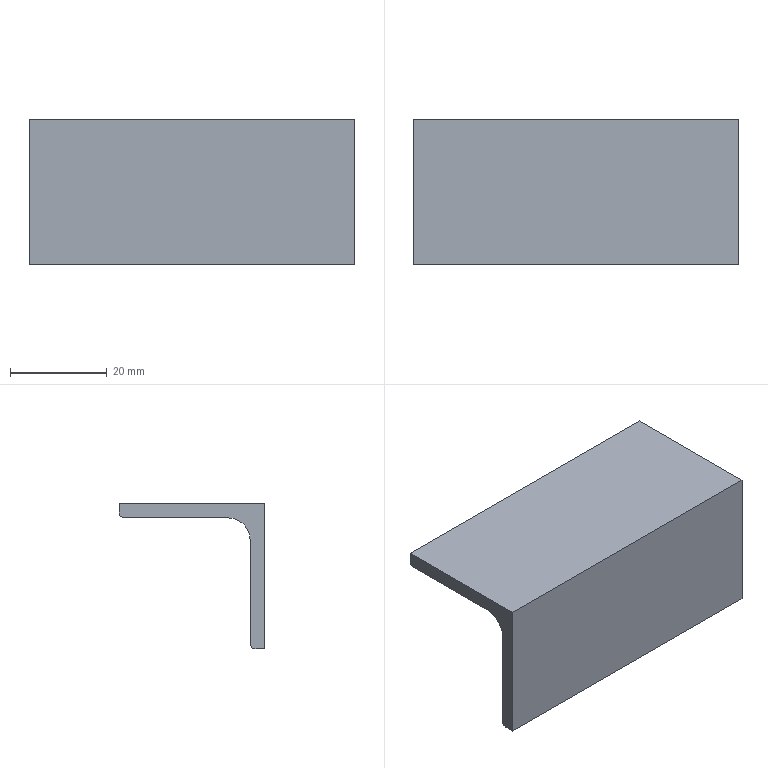Part | STEP file | 02-Angle steel 30x30x3_default<machining> | 1 solid | 11 faces | box 67 x 30 x 30 mm | volume 11719 mm3 | plane 8 | cylinder 3 | commonest cylinder face diameters 2 x2 9 x1
STEP:
#1=CARTESIAN_POINT('',(0.,0.,0.));
#2=DIRECTION('',(0.,0.,1.));
#3=DIRECTION('',(1.,0.,0.));
#4=AXIS2_PLACEMENT_3D('',#1,#2,#3);
#5=CARTESIAN_POINT('',(0.,30.,-2.));
#6=VERTEX_POINT('',#5);
#7=CARTESIAN_POINT('',(0.,30.,0.));
#8=VERTEX_POINT('',#7);
#9=CARTESIAN_POINT('',(0.,30.,0.));
#10=DIRECTION('',(0.,0.,1.));
#11=VECTOR('',#10,1.);
#12=LINE('',#9,#11);
#13=CARTESIAN_POINT('',(67.,30.,0.));
#14=DIRECTION('',(0.,-1.,0.));
#15=DIRECTION('',(0.,0.,-1.));
#16=AXIS2_PLACEMENT_3D('',#13,#14,#15);
#17=PLANE('',#16);
#18=CARTESIAN_POINT('',(0.,-67.));
#19=DIRECTION('',(-1.,0.));
#20=VECTOR('',#19,1.);
#21=LINE('',#18,#20);
#22=(GEOMETRIC_REPRESENTATION_CONTEXT(2)PARAMETRIC_REPRESENTATION_CONTEXT()REPRESENTATION_CONTEXT('',''));
#23=DEFINITIONAL_REPRESENTATION('',(#21),#22);
#24=PCURVE('',#17,#23);
#25=CARTESIAN_POINT('',(0.,29.,-2.));
#26=DIRECTION('',(-1.,0.,0.));
#27=DIRECTION('',(0.,0.,1.));
#28=AXIS2_PLACEMENT_3D('',#25,#26,#27);
#29=PLANE('',#28);
#30=CARTESIAN_POINT('',(2.,1.));
#31=DIRECTION('',(1.,0.));
#32=VECTOR('',#31,1.);
#33=LINE('',#30,#32);
#34=(GEOMETRIC_REPRESENTATION_CONTEXT(2)PARAMETRIC_REPRESENTATION_CONTEXT()REPRESENTATION_CONTEXT('',''));
#35=DEFINITIONAL_REPRESENTATION('',(#33),#34);
#36=PCURVE('',#29,#35);
#37=SURFACE_CURVE('',#12,(#24,#36),.PCURVE_S1.);
#38=EDGE_CURVE('',#6,#8,#37,.T.);
#39=ORIENTED_EDGE('',*,*,#38,.T.);
#40=CARTESIAN_POINT('',(67.,30.,0.));
#41=VERTEX_POINT('',#40);
#42=CARTESIAN_POINT('',(67.,30.,0.));
#43=DIRECTION('',(-1.,0.,0.));
#44=VECTOR('',#43,1.);
#45=LINE('',#42,#44);
#46=CARTESIAN_POINT('',(0.,0.));
#47=DIRECTION('',(0.,-1.));
#48=VECTOR('',#47,1.);
#49=LINE('',#46,#48);
#50=(GEOMETRIC_REPRESENTATION_CONTEXT(2)PARAMETRIC_REPRESENTATION_CONTEXT()REPRESENTATION_CONTEXT('',''));
#51=DEFINITIONAL_REPRESENTATION('',(#49),#50);
#52=PCURVE('',#17,#51);
#53=CARTESIAN_POINT('',(67.,30.,0.));
#54=DIRECTION('',(0.,0.,-1.));
#55=DIRECTION('',(0.,1.,0.));
#56=AXIS2_PLACEMENT_3D('',#53,#54,#55);
#57=PLANE('',#56);
#58=CARTESIAN_POINT('',(0.,0.));
#59=DIRECTION('',(0.,-1.));
#60=VECTOR('',#59,1.);
#61=LINE('',#58,#60);
#62=(GEOMETRIC_REPRESENTATION_CONTEXT(2)PARAMETRIC_REPRESENTATION_CONTEXT()REPRESENTATION_CONTEXT('',''));
#63=DEFINITIONAL_REPRESENTATION('',(#61),#62);
#64=PCURVE('',#57,#63);
#65=SURFACE_CURVE('',#45,(#52,#64),.PCURVE_S1.);
#66=EDGE_CURVE('',#41,#8,#65,.T.);
#67=ORIENTED_EDGE('',*,*,#66,.F.);
#68=CARTESIAN_POINT('',(67.,30.,-2.));
#69=VERTEX_POINT('',#68);
#70=CARTESIAN_POINT('',(67.,30.,0.));
#71=DIRECTION('',(0.,0.,1.));
#72=VECTOR('',#71,1.);
#73=LINE('',#70,#72);
#74=CARTESIAN_POINT('',(0.,0.));
#75=DIRECTION('',(-1.,0.));
#76=VECTOR('',#75,1.);
#77=LINE('',#74,#76);
#78=(GEOMETRIC_REPRESENTATION_CONTEXT(2)PARAMETRIC_REPRESENTATION_CONTEXT()REPRESENTATION_CONTEXT('',''));
#79=DEFINITIONAL_REPRESENTATION('',(#77),#78);
#80=PCURVE('',#17,#79);
#81=CARTESIAN_POINT('',(67.,29.,-2.));
#82=DIRECTION('',(-1.,0.,0.));
#83=DIRECTION('',(0.,0.,1.));
#84=AXIS2_PLACEMENT_3D('',#81,#82,#83);
#85=PLANE('',#84);
#86=CARTESIAN_POINT('',(2.,1.));
#87=DIRECTION('',(1.,0.));
#88=VECTOR('',#87,1.);
#89=LINE('',#86,#88);
#90=(GEOMETRIC_REPRESENTATION_CONTEXT(2)PARAMETRIC_REPRESENTATION_CONTEXT()REPRESENTATION_CONTEXT('',''));
#91=DEFINITIONAL_REPRESENTATION('',(#89),#90);
#92=PCURVE('',#85,#91);
#93=SURFACE_CURVE('',#73,(#80,#92),.PCURVE_S1.);
#94=EDGE_CURVE('',#69,#41,#93,.T.);
#95=ORIENTED_EDGE('',*,*,#94,.F.);
#96=CARTESIAN_POINT('',(67.,30.,-2.));
#97=DIRECTION('',(-1.,0.,0.));
#98=VECTOR('',#97,1.);
#99=LINE('',#96,#98);
#100=CARTESIAN_POINT('',(2.,0.));
#101=DIRECTION('',(0.,-1.));
#102=VECTOR('',#101,1.);
#103=LINE('',#100,#102);
#104=(GEOMETRIC_REPRESENTATION_CONTEXT(2)PARAMETRIC_REPRESENTATION_CONTEXT()REPRESENTATION_CONTEXT('',''));
#105=DEFINITIONAL_REPRESENTATION('',(#103),#104);
#106=PCURVE('',#17,#105);
#107=CARTESIAN_POINT('',(67.,29.,-2.));
#108=DIRECTION('',(-1.,0.,0.));
#109=DIRECTION('',(0.,0.,1.));
#110=AXIS2_PLACEMENT_3D('',#107,#108,#109);
#111=CYLINDRICAL_SURFACE('',#110,1.);
#112=CARTESIAN_POINT('',(1.571,0.));
#113=DIRECTION('',(0.,1.));
#114=VECTOR('',#113,1.);
#115=LINE('',#112,#114);
#116=(GEOMETRIC_REPRESENTATION_CONTEXT(2)PARAMETRIC_REPRESENTATION_CONTEXT()REPRESENTATION_CONTEXT('',''));
#117=DEFINITIONAL_REPRESENTATION('',(#115),#116);
#118=PCURVE('',#111,#117);
#119=SURFACE_CURVE('',#99,(#106,#118),.PCURVE_S1.);
#120=EDGE_CURVE('',#69,#6,#119,.T.);
#121=ORIENTED_EDGE('',*,*,#120,.T.);
#122=EDGE_LOOP('',(#39,#67,#95,#121));
#123=FACE_BOUND('',#122,.T.);
#124=ADVANCED_FACE('',(#123),#17,.F.);
#125=CARTESIAN_POINT('',(0.,0.,0.));
#126=VERTEX_POINT('',#125);
#127=CARTESIAN_POINT('',(0.,30.,0.));
#128=DIRECTION('',(0.,-1.,0.));
#129=VECTOR('',#128,1.);
#130=LINE('',#127,#129);
#131=CARTESIAN_POINT('',(0.,-67.));
#132=DIRECTION('',(-1.,0.));
#133=VECTOR('',#132,1.);
#134=LINE('',#131,#133);
#135=(GEOMETRIC_REPRESENTATION_CONTEXT(2)PARAMETRIC_REPRESENTATION_CONTEXT()REPRESENTATION_CONTEXT('',''));
#136=DEFINITIONAL_REPRESENTATION('',(#134),#135);
#137=PCURVE('',#57,#136);
#138=CARTESIAN_POINT('',(2.,1.));
#139=DIRECTION('',(0.,-1.));
#140=VECTOR('',#139,1.);
#141=LINE('',#138,#140);
#142=(GEOMETRIC_REPRESENTATION_CONTEXT(2)PARAMETRIC_REPRESENTATION_CONTEXT()REPRESENTATION_CONTEXT('',''));
#143=DEFINITIONAL_REPRESENTATION('',(#141),#142);
#144=PCURVE('',#29,#143);
#145=SURFACE_CURVE('',#130,(#137,#144),.PCURVE_S1.);
#146=EDGE_CURVE('',#8,#126,#145,.T.);
#147=ORIENTED_EDGE('',*,*,#146,.T.);
#148=CARTESIAN_POINT('',(67.,0.,0.));
#149=VERTEX_POINT('',#148);
#150=CARTESIAN_POINT('',(67.,0.,0.));
#151=DIRECTION('',(-1.,0.,0.));
#152=VECTOR('',#151,1.);
#153=LINE('',#150,#152);
#154=CARTESIAN_POINT('',(-30.,0.));
#155=DIRECTION('',(0.,-1.));
#156=VECTOR('',#155,1.);
#157=LINE('',#154,#156);
#158=(GEOMETRIC_REPRESENTATION_CONTEXT(2)PARAMETRIC_REPRESENTATION_CONTEXT()REPRESENTATION_CONTEXT('',''));
#159=DEFINITIONAL_REPRESENTATION('',(#157),#158);
#160=PCURVE('',#57,#159);
#161=CARTESIAN_POINT('',(67.,0.,0.));
#162=DIRECTION('',(0.,1.,0.));
#163=DIRECTION('',(0.,0.,1.));
#164=AXIS2_PLACEMENT_3D('',#161,#162,#163);
#165=PLANE('',#164);
#166=CARTESIAN_POINT('',(0.,0.));
#167=DIRECTION('',(0.,-1.));
#168=VECTOR('',#167,1.);
#169=LINE('',#166,#168);
#170=(GEOMETRIC_REPRESENTATION_CONTEXT(2)PARAMETRIC_REPRESENTATION_CONTEXT()REPRESENTATION_CONTEXT('',''));
#171=DEFINITIONAL_REPRESENTATION('',(#169),#170);
#172=PCURVE('',#165,#171);
#173=SURFACE_CURVE('',#153,(#160,#172),.PCURVE_S1.);
#174=EDGE_CURVE('',#149,#126,#173,.T.);
#175=ORIENTED_EDGE('',*,*,#174,.F.);
#176=CARTESIAN_POINT('',(67.,30.,0.));
#177=DIRECTION('',(0.,-1.,0.));
#178=VECTOR('',#177,1.);
#179=LINE('',#176,#178);
#180=CARTESIAN_POINT('',(0.,0.));
#181=DIRECTION('',(-1.,0.));
#182=VECTOR('',#181,1.);
#183=LINE('',#180,#182);
#184=(GEOMETRIC_REPRESENTATION_CONTEXT(2)PARAMETRIC_REPRESENTATION_CONTEXT()REPRESENTATION_CONTEXT('',''));
#185=DEFINITIONAL_REPRESENTATION('',(#183),#184);
#186=PCURVE('',#57,#185);
#187=CARTESIAN_POINT('',(2.,1.));
#188=DIRECTION('',(0.,-1.));
#189=VECTOR('',#188,1.);
#190=LINE('',#187,#189);
#191=(GEOMETRIC_REPRESENTATION_CONTEXT(2)PARAMETRIC_REPRESENTATION_CONTEXT()REPRESENTATION_CONTEXT('',''));
#192=DEFINITIONAL_REPRESENTATION('',(#190),#191);
#193=PCURVE('',#85,#192);
#194=SURFACE_CURVE('',#179,(#186,#193),.PCURVE_S1.);
#195=EDGE_CURVE('',#41,#149,#194,.T.);
#196=ORIENTED_EDGE('',*,*,#195,.F.);
#197=ORIENTED_EDGE('',*,*,#66,.T.);
#198=EDGE_LOOP('',(#147,#175,#196,#197));
#199=FACE_BOUND('',#198,.T.);
#200=ADVANCED_FACE('',(#199),#57,.F.);
#201=CARTESIAN_POINT('',(0.,0.,-30.));
#202=VERTEX_POINT('',#201);
#203=CARTESIAN_POINT('',(0.,0.,0.));
#204=DIRECTION('',(0.,0.,-1.));
#205=VECTOR('',#204,1.);
#206=LINE('',#203,#205);
#207=CARTESIAN_POINT('',(0.,-67.));
#208=DIRECTION('',(-1.,0.));
#209=VECTOR('',#208,1.);
#210=LINE('',#207,#209);
#211=(GEOMETRIC_REPRESENTATION_CONTEXT(2)PARAMETRIC_REPRESENTATION_CONTEXT()REPRESENTATION_CONTEXT('',''));
#212=DEFINITIONAL_REPRESENTATION('',(#210),#211);
#213=PCURVE('',#165,#212);
#214=CARTESIAN_POINT('',(2.,-29.));
#215=DIRECTION('',(-1.,0.));
#216=VECTOR('',#215,1.);
#217=LINE('',#214,#216);
#218=(GEOMETRIC_REPRESENTATION_CONTEXT(2)PARAMETRIC_REPRESENTATION_CONTEXT()REPRESENTATION_CONTEXT('',''));
#219=DEFINITIONAL_REPRESENTATION('',(#217),#218);
#220=PCURVE('',#29,#219);
#221=SURFACE_CURVE('',#206,(#213,#220),.PCURVE_S1.);
#222=EDGE_CURVE('',#126,#202,#221,.T.);
#223=ORIENTED_EDGE('',*,*,#222,.T.);
#224=CARTESIAN_POINT('',(67.,0.,-30.));
#225=VERTEX_POINT('',#224);
#226=CARTESIAN_POINT('',(67.,0.,-30.));
#227=DIRECTION('',(-1.,0.,0.));
#228=VECTOR('',#227,1.);
#229=LINE('',#226,#228);
#230=CARTESIAN_POINT('',(-30.,0.));
#231=DIRECTION('',(0.,-1.));
#232=VECTOR('',#231,1.);
#233=LINE('',#230,#232);
#234=(GEOMETRIC_REPRESENTATION_CONTEXT(2)PARAMETRIC_REPRESENTATION_CONTEXT()REPRESENTATION_CONTEXT('',''));
#235=DEFINITIONAL_REPRESENTATION('',(#233),#234);
#236=PCURVE('',#165,#235);
#237=CARTESIAN_POINT('',(67.,0.,-30.));
#238=DIRECTION('',(0.,0.,1.));
#239=DIRECTION('',(0.,-1.,0.));
#240=AXIS2_PLACEMENT_3D('',#237,#238,#239);
#241=PLANE('',#240);
#242=CARTESIAN_POINT('',(0.,0.));
#243=DIRECTION('',(0.,-1.));
#244=VECTOR('',#243,1.);
#245=LINE('',#242,#244);
#246=(GEOMETRIC_REPRESENTATION_CONTEXT(2)PARAMETRIC_REPRESENTATION_CONTEXT()REPRESENTATION_CONTEXT('',''));
#247=DEFINITIONAL_REPRESENTATION('',(#245),#246);
#248=PCURVE('',#241,#247);
#249=SURFACE_CURVE('',#229,(#236,#248),.PCURVE_S1.);
#250=EDGE_CURVE('',#225,#202,#249,.T.);
#251=ORIENTED_EDGE('',*,*,#250,.F.);
#252=CARTESIAN_POINT('',(67.,0.,0.));
#253=DIRECTION('',(0.,0.,-1.));
#254=VECTOR('',#253,1.);
#255=LINE('',#252,#254);
#256=CARTESIAN_POINT('',(0.,0.));
#257=DIRECTION('',(-1.,0.));
#258=VECTOR('',#257,1.);
#259=LINE('',#256,#258);
#260=(GEOMETRIC_REPRESENTATION_CONTEXT(2)PARAMETRIC_REPRESENTATION_CONTEXT()REPRESENTATION_CONTEXT('',''));
#261=DEFINITIONAL_REPRESENTATION('',(#259),#260);
#262=PCURVE('',#165,#261);
#263=CARTESIAN_POINT('',(2.,-29.));
#264=DIRECTION('',(-1.,0.));
#265=VECTOR('',#264,1.);
#266=LINE('',#263,#265);
#267=(GEOMETRIC_REPRESENTATION_CONTEXT(2)PARAMETRIC_REPRESENTATION_CONTEXT()REPRESENTATION_CONTEXT('',''));
#268=DEFINITIONAL_REPRESENTATION('',(#266),#267);
#269=PCURVE('',#85,#268);
#270=SURFACE_CURVE('',#255,(#262,#269),.PCURVE_S1.);
#271=EDGE_CURVE('',#149,#225,#270,.T.);
#272=ORIENTED_EDGE('',*,*,#271,.F.);
#273=ORIENTED_EDGE('',*,*,#174,.T.);
#274=EDGE_LOOP('',(#223,#251,#272,#273));
#275=FACE_BOUND('',#274,.T.);
#276=ADVANCED_FACE('',(#275),#165,.F.);
#277=CARTESIAN_POINT('',(0.,2.,-30.));
#278=VERTEX_POINT('',#277);
#279=CARTESIAN_POINT('',(0.,0.,-30.));
#280=DIRECTION('',(0.,1.,0.));
#281=VECTOR('',#280,1.);
#282=LINE('',#279,#281);
#283=CARTESIAN_POINT('',(0.,-67.));
#284=DIRECTION('',(-1.,0.));
#285=VECTOR('',#284,1.);
#286=LINE('',#283,#285);
#287=(GEOMETRIC_REPRESENTATION_CONTEXT(2)PARAMETRIC_REPRESENTATION_CONTEXT()REPRESENTATION_CONTEXT('',''));
#288=DEFINITIONAL_REPRESENTATION('',(#286),#287);
#289=PCURVE('',#241,#288);
#290=CARTESIAN_POINT('',(-28.,-29.));
#291=DIRECTION('',(0.,1.));
#292=VECTOR('',#291,1.);
#293=LINE('',#290,#292);
#294=(GEOMETRIC_REPRESENTATION_CONTEXT(2)PARAMETRIC_REPRESENTATION_CONTEXT()REPRESENTATION_CONTEXT('',''));
#295=DEFINITIONAL_REPRESENTATION('',(#293),#294);
#296=PCURVE('',#29,#295);
#297=SURFACE_CURVE('',#282,(#289,#296),.PCURVE_S1.);
#298=EDGE_CURVE('',#202,#278,#297,.T.);
#299=ORIENTED_EDGE('',*,*,#298,.T.);
#300=CARTESIAN_POINT('',(67.,2.,-30.));
#301=VERTEX_POINT('',#300);
#302=CARTESIAN_POINT('',(67.,2.,-30.));
#303=DIRECTION('',(-1.,0.,0.));
#304=VECTOR('',#303,1.);
#305=LINE('',#302,#304);
#306=CARTESIAN_POINT('',(-2.,0.));
#307=DIRECTION('',(0.,-1.));
#308=VECTOR('',#307,1.);
#309=LINE('',#306,#308);
#310=(GEOMETRIC_REPRESENTATION_CONTEXT(2)PARAMETRIC_REPRESENTATION_CONTEXT()REPRESENTATION_CONTEXT('',''));
#311=DEFINITIONAL_REPRESENTATION('',(#309),#310);
#312=PCURVE('',#241,#311);
#313=CARTESIAN_POINT('',(67.,2.,-29.));
#314=DIRECTION('',(-1.,0.,0.));
#315=DIRECTION('',(0.,0.,1.));
#316=AXIS2_PLACEMENT_3D('',#313,#314,#315);
#317=CYLINDRICAL_SURFACE('',#316,1.);
#318=CARTESIAN_POINT('',(3.142,0.));
#319=DIRECTION('',(0.,1.));
#320=VECTOR('',#319,1.);
#321=LINE('',#318,#320);
#322=(GEOMETRIC_REPRESENTATION_CONTEXT(2)PARAMETRIC_REPRESENTATION_CONTEXT()REPRESENTATION_CONTEXT('',''));
#323=DEFINITIONAL_REPRESENTATION('',(#321),#322);
#324=PCURVE('',#317,#323);
#325=SURFACE_CURVE('',#305,(#312,#324),.PCURVE_S1.);
#326=EDGE_CURVE('',#301,#278,#325,.T.);
#327=ORIENTED_EDGE('',*,*,#326,.F.);
#328=CARTESIAN_POINT('',(67.,0.,-30.));
#329=DIRECTION('',(0.,1.,0.));
#330=VECTOR('',#329,1.);
#331=LINE('',#328,#330);
#332=CARTESIAN_POINT('',(0.,0.));
#333=DIRECTION('',(-1.,0.));
#334=VECTOR('',#333,1.);
#335=LINE('',#332,#334);
#336=(GEOMETRIC_REPRESENTATION_CONTEXT(2)PARAMETRIC_REPRESENTATION_CONTEXT()REPRESENTATION_CONTEXT('',''));
#337=DEFINITIONAL_REPRESENTATION('',(#335),#336);
#338=PCURVE('',#241,#337);
#339=CARTESIAN_POINT('',(-28.,-29.));
#340=DIRECTION('',(0.,1.));
#341=VECTOR('',#340,1.);
#342=LINE('',#339,#341);
#343=(GEOMETRIC_REPRESENTATION_CONTEXT(2)PARAMETRIC_REPRESENTATION_CONTEXT()REPRESENTATION_CONTEXT('',''));
#344=DEFINITIONAL_REPRESENTATION('',(#342),#343);
#345=PCURVE('',#85,#344);
#346=SURFACE_CURVE('',#331,(#338,#345),.PCURVE_S1.);
#347=EDGE_CURVE('',#225,#301,#346,.T.);
#348=ORIENTED_EDGE('',*,*,#347,.F.);
#349=ORIENTED_EDGE('',*,*,#250,.T.);
#350=EDGE_LOOP('',(#299,#327,#348,#349));
#351=FACE_BOUND('',#350,.T.);
#352=ADVANCED_FACE('',(#351),#241,.F.);
#353=CARTESIAN_POINT('',(0.,3.,-29.));
#354=VERTEX_POINT('',#353);
#355=CARTESIAN_POINT('',(0.,2.,-29.));
#356=DIRECTION('',(1.,0.,0.));
#357=DIRECTION('',(0.,0.,-1.));
#358=AXIS2_PLACEMENT_3D('',#355,#356,#357);
#359=CIRCLE('',#358,1.);
#360=CARTESIAN_POINT('',(3.142,67.));
#361=DIRECTION('',(-1.,0.));
#362=VECTOR('',#361,1.);
#363=LINE('',#360,#362);
#364=(GEOMETRIC_REPRESENTATION_CONTEXT(2)PARAMETRIC_REPRESENTATION_CONTEXT()REPRESENTATION_CONTEXT('',''));
#365=DEFINITIONAL_REPRESENTATION('',(#363),#364);
#366=PCURVE('',#317,#365);
#367=CARTESIAN_POINT('',(-28.,-27.));
#368=CARTESIAN_POINT('',(-28.,-25.268));
#369=CARTESIAN_POINT('',(-26.5,-26.134));
#370=CARTESIAN_POINT('',(-25.,-27.));
#371=CARTESIAN_POINT('',(-26.5,-27.866));
#372=CARTESIAN_POINT('',(-28.,-28.732));
#373=CARTESIAN_POINT('',(-28.,-27.));
#374=(BOUNDED_CURVE()B_SPLINE_CURVE(2,(#367,#368,#369,#370,#371,#372,#373),.UNSPECIFIED.,.T.,.F.)B_SPLINE_CURVE_WITH_KNOTS((1,2,2,2,2,1),(-2.094,0.,2.094,4.189,6.283,8.378),.UNSPECIFIED.)CURVE()GEOMETRIC_REPRESENTATION_ITEM()RATIONAL_B_SPLINE_CURVE((1.,0.5,1.,0.5,1.,0.5,1.))REPRESENTATION_ITEM(''));
#375=(GEOMETRIC_REPRESENTATION_CONTEXT(2)PARAMETRIC_REPRESENTATION_CONTEXT()REPRESENTATION_CONTEXT('',''));
#376=DEFINITIONAL_REPRESENTATION('',(#374),#375);
#377=PCURVE('',#29,#376);
#378=SURFACE_CURVE('',#359,(#366,#377),.PCURVE_S1.);
#379=EDGE_CURVE('',#278,#354,#378,.T.);
#380=ORIENTED_EDGE('',*,*,#379,.T.);
#381=CARTESIAN_POINT('',(67.,3.,-29.));
#382=VERTEX_POINT('',#381);
#383=CARTESIAN_POINT('',(67.,3.,-29.));
#384=DIRECTION('',(-1.,0.,0.));
#385=VECTOR('',#384,1.);
#386=LINE('',#383,#385);
#387=CARTESIAN_POINT('',(1.571,0.));
#388=DIRECTION('',(0.,1.));
#389=VECTOR('',#388,1.);
#390=LINE('',#387,#389);
#391=(GEOMETRIC_REPRESENTATION_CONTEXT(2)PARAMETRIC_REPRESENTATION_CONTEXT()REPRESENTATION_CONTEXT('',''));
#392=DEFINITIONAL_REPRESENTATION('',(#390),#391);
#393=PCURVE('',#317,#392);
#394=CARTESIAN_POINT('',(67.,3.,-7.5));
#395=DIRECTION('',(0.,-1.,0.));
#396=DIRECTION('',(0.,0.,-1.));
#397=AXIS2_PLACEMENT_3D('',#394,#395,#396);
#398=PLANE('',#397);
#399=CARTESIAN_POINT('',(21.5,0.));
#400=DIRECTION('',(0.,-1.));
#401=VECTOR('',#400,1.);
#402=LINE('',#399,#401);
#403=(GEOMETRIC_REPRESENTATION_CONTEXT(2)PARAMETRIC_REPRESENTATION_CONTEXT()REPRESENTATION_CONTEXT('',''));
#404=DEFINITIONAL_REPRESENTATION('',(#402),#403);
#405=PCURVE('',#398,#404);
#406=SURFACE_CURVE('',#386,(#393,#405),.PCURVE_S1.);
#407=EDGE_CURVE('',#382,#354,#406,.T.);
#408=ORIENTED_EDGE('',*,*,#407,.F.);
#409=CARTESIAN_POINT('',(67.,2.,-29.));
#410=DIRECTION('',(1.,0.,0.));
#411=DIRECTION('',(0.,0.,-1.));
#412=AXIS2_PLACEMENT_3D('',#409,#410,#411);
#413=CIRCLE('',#412,1.);
#414=CARTESIAN_POINT('',(3.142,0.));
#415=DIRECTION('',(-1.,0.));
#416=VECTOR('',#415,1.);
#417=LINE('',#414,#416);
#418=(GEOMETRIC_REPRESENTATION_CONTEXT(2)PARAMETRIC_REPRESENTATION_CONTEXT()REPRESENTATION_CONTEXT('',''));
#419=DEFINITIONAL_REPRESENTATION('',(#417),#418);
#420=PCURVE('',#317,#419);
#421=CARTESIAN_POINT('',(-28.,-27.));
#422=CARTESIAN_POINT('',(-28.,-25.268));
#423=CARTESIAN_POINT('',(-26.5,-26.134));
#424=CARTESIAN_POINT('',(-25.,-27.));
#425=CARTESIAN_POINT('',(-26.5,-27.866));
#426=CARTESIAN_POINT('',(-28.,-28.732));
#427=CARTESIAN_POINT('',(-28.,-27.));
#428=(BOUNDED_CURVE()B_SPLINE_CURVE(2,(#421,#422,#423,#424,#425,#426,#427),.UNSPECIFIED.,.T.,.F.)B_SPLINE_CURVE_WITH_KNOTS((1,2,2,2,2,1),(-2.094,0.,2.094,4.189,6.283,8.378),.UNSPECIFIED.)CURVE()GEOMETRIC_REPRESENTATION_ITEM()RATIONAL_B_SPLINE_CURVE((1.,0.5,1.,0.5,1.,0.5,1.))REPRESENTATION_ITEM(''));
#429=(GEOMETRIC_REPRESENTATION_CONTEXT(2)PARAMETRIC_REPRESENTATION_CONTEXT()REPRESENTATION_CONTEXT('',''));
#430=DEFINITIONAL_REPRESENTATION('',(#428),#429);
#431=PCURVE('',#85,#430);
#432=SURFACE_CURVE('',#413,(#420,#431),.PCURVE_S1.);
#433=EDGE_CURVE('',#301,#382,#432,.T.);
#434=ORIENTED_EDGE('',*,*,#433,.F.);
#435=ORIENTED_EDGE('',*,*,#326,.T.);
#436=EDGE_LOOP('',(#380,#408,#434,#435));
#437=FACE_BOUND('',#436,.T.);
#438=ADVANCED_FACE('',(#437),#317,.T.);
#439=CARTESIAN_POINT('',(0.,3.,-7.5));
#440=VERTEX_POINT('',#439);
#441=CARTESIAN_POINT('',(0.,3.,-7.5));
#442=DIRECTION('',(0.,0.,1.));
#443=VECTOR('',#442,1.);
#444=LINE('',#441,#443);
#445=CARTESIAN_POINT('',(0.,-67.));
#446=DIRECTION('',(-1.,0.));
#447=VECTOR('',#446,1.);
#448=LINE('',#445,#447);
#449=(GEOMETRIC_REPRESENTATION_CONTEXT(2)PARAMETRIC_REPRESENTATION_CONTEXT()REPRESENTATION_CONTEXT('',''));
#450=DEFINITIONAL_REPRESENTATION('',(#448),#449);
#451=PCURVE('',#398,#450);
#452=CARTESIAN_POINT('',(-5.5,-26.));
#453=DIRECTION('',(1.,0.));
#454=VECTOR('',#453,1.);
#455=LINE('',#452,#454);
#456=(GEOMETRIC_REPRESENTATION_CONTEXT(2)PARAMETRIC_REPRESENTATION_CONTEXT()REPRESENTATION_CONTEXT('',''));
#457=DEFINITIONAL_REPRESENTATION('',(#455),#456);
#458=PCURVE('',#29,#457);
#459=SURFACE_CURVE('',#444,(#451,#458),.PCURVE_S1.);
#460=EDGE_CURVE('',#354,#440,#459,.T.);
#461=ORIENTED_EDGE('',*,*,#460,.T.);
#462=CARTESIAN_POINT('',(67.,3.,-7.5));
#463=VERTEX_POINT('',#462);
#464=CARTESIAN_POINT('',(67.,3.,-7.5));
#465=DIRECTION('',(-1.,0.,0.));
#466=VECTOR('',#465,1.);
#467=LINE('',#464,#466);
#468=CARTESIAN_POINT('',(0.,0.));
#469=DIRECTION('',(0.,-1.));
#470=VECTOR('',#469,1.);
#471=LINE('',#468,#470);
#472=(GEOMETRIC_REPRESENTATION_CONTEXT(2)PARAMETRIC_REPRESENTATION_CONTEXT()REPRESENTATION_CONTEXT('',''));
#473=DEFINITIONAL_REPRESENTATION('',(#471),#472);
#474=PCURVE('',#398,#473);
#475=CARTESIAN_POINT('',(67.,7.5,-7.5));
#476=DIRECTION('',(-1.,0.,0.));
#477=DIRECTION('',(0.,0.,1.));
#478=AXIS2_PLACEMENT_3D('',#475,#476,#477);
#479=CYLINDRICAL_SURFACE('',#478,4.5);
#480=CARTESIAN_POINT('',(4.712,0.));
#481=DIRECTION('',(0.,1.));
#482=VECTOR('',#481,1.);
#483=LINE('',#480,#482);
#484=(GEOMETRIC_REPRESENTATION_CONTEXT(2)PARAMETRIC_REPRESENTATION_CONTEXT()REPRESENTATION_CONTEXT('',''));
#485=DEFINITIONAL_REPRESENTATION('',(#483),#484);
#486=PCURVE('',#479,#485);
#487=SURFACE_CURVE('',#467,(#474,#486),.PCURVE_S1.);
#488=EDGE_CURVE('',#463,#440,#487,.T.);
#489=ORIENTED_EDGE('',*,*,#488,.F.);
#490=CARTESIAN_POINT('',(67.,3.,-7.5));
#491=DIRECTION('',(0.,0.,1.));
#492=VECTOR('',#491,1.);
#493=LINE('',#490,#492);
#494=CARTESIAN_POINT('',(0.,0.));
#495=DIRECTION('',(-1.,0.));
#496=VECTOR('',#495,1.);
#497=LINE('',#494,#496);
#498=(GEOMETRIC_REPRESENTATION_CONTEXT(2)PARAMETRIC_REPRESENTATION_CONTEXT()REPRESENTATION_CONTEXT('',''));
#499=DEFINITIONAL_REPRESENTATION('',(#497),#498);
#500=PCURVE('',#398,#499);
#501=CARTESIAN_POINT('',(-5.5,-26.));
#502=DIRECTION('',(1.,0.));
#503=VECTOR('',#502,1.);
#504=LINE('',#501,#503);
#505=(GEOMETRIC_REPRESENTATION_CONTEXT(2)PARAMETRIC_REPRESENTATION_CONTEXT()REPRESENTATION_CONTEXT('',''));
#506=DEFINITIONAL_REPRESENTATION('',(#504),#505);
#507=PCURVE('',#85,#506);
#508=SURFACE_CURVE('',#493,(#500,#507),.PCURVE_S1.);
#509=EDGE_CURVE('',#382,#463,#508,.T.);
#510=ORIENTED_EDGE('',*,*,#509,.F.);
#511=ORIENTED_EDGE('',*,*,#407,.T.);
#512=EDGE_LOOP('',(#461,#489,#510,#511));
#513=FACE_BOUND('',#512,.T.);
#514=ADVANCED_FACE('',(#513),#398,.F.);
#515=ORIENTED_EDGE('',*,*,#488,.F.);
#516=CARTESIAN_POINT('',(67.,7.5,-3.));
#517=VERTEX_POINT('',#516);
#518=CARTESIAN_POINT('',(67.,7.5,-7.5));
#519=DIRECTION('',(-1.,0.,0.));
#520=DIRECTION('',(0.,0.,-1.));
#521=AXIS2_PLACEMENT_3D('',#518,#519,#520);
#522=CIRCLE('',#521,4.5);
#523=CARTESIAN_POINT('',(3.142,0.));
#524=DIRECTION('',(1.,0.));
#525=VECTOR('',#524,1.);
#526=LINE('',#523,#525);
#527=(GEOMETRIC_REPRESENTATION_CONTEXT(2)PARAMETRIC_REPRESENTATION_CONTEXT()REPRESENTATION_CONTEXT('',''));
#528=DEFINITIONAL_REPRESENTATION('',(#526),#527);
#529=PCURVE('',#479,#528);
#530=CARTESIAN_POINT('',(-5.5,-21.5));
#531=DIRECTION('',(-1.,0.));
#532=AXIS2_PLACEMENT_2D('',#530,#531);
#533=CIRCLE('',#532,4.5);
#534=(GEOMETRIC_REPRESENTATION_CONTEXT(2)PARAMETRIC_REPRESENTATION_CONTEXT()REPRESENTATION_CONTEXT('',''));
#535=DEFINITIONAL_REPRESENTATION('',(#533),#534);
#536=PCURVE('',#85,#535);
#537=SURFACE_CURVE('',#522,(#529,#536),.PCURVE_S1.);
#538=EDGE_CURVE('',#463,#517,#537,.T.);
#539=ORIENTED_EDGE('',*,*,#538,.T.);
#540=CARTESIAN_POINT('',(0.,7.5,-3.));
#541=VERTEX_POINT('',#540);
#542=CARTESIAN_POINT('',(67.,7.5,-3.));
#543=DIRECTION('',(-1.,0.,0.));
#544=VECTOR('',#543,1.);
#545=LINE('',#542,#544);
#546=CARTESIAN_POINT('',(6.283,0.));
#547=DIRECTION('',(0.,1.));
#548=VECTOR('',#547,1.);
#549=LINE('',#546,#548);
#550=(GEOMETRIC_REPRESENTATION_CONTEXT(2)PARAMETRIC_REPRESENTATION_CONTEXT()REPRESENTATION_CONTEXT('',''));
#551=DEFINITIONAL_REPRESENTATION('',(#549),#550);
#552=PCURVE('',#479,#551);
#553=CARTESIAN_POINT('',(67.,29.,-3.));
#554=DIRECTION('',(0.,0.,1.));
#555=DIRECTION('',(0.,-1.,0.));
#556=AXIS2_PLACEMENT_3D('',#553,#554,#555);
#557=PLANE('',#556);
#558=CARTESIAN_POINT('',(21.5,0.));
#559=DIRECTION('',(0.,-1.));
#560=VECTOR('',#559,1.);
#561=LINE('',#558,#560);
#562=(GEOMETRIC_REPRESENTATION_CONTEXT(2)PARAMETRIC_REPRESENTATION_CONTEXT()REPRESENTATION_CONTEXT('',''));
#563=DEFINITIONAL_REPRESENTATION('',(#561),#562);
#564=PCURVE('',#557,#563);
#565=SURFACE_CURVE('',#545,(#552,#564),.PCURVE_S1.);
#566=EDGE_CURVE('',#517,#541,#565,.T.);
#567=ORIENTED_EDGE('',*,*,#566,.T.);
#568=CARTESIAN_POINT('',(0.,7.5,-7.5));
#569=DIRECTION('',(-1.,0.,0.));
#570=DIRECTION('',(0.,0.,-1.));
#571=AXIS2_PLACEMENT_3D('',#568,#569,#570);
#572=CIRCLE('',#571,4.5);
#573=CARTESIAN_POINT('',(3.142,67.));
#574=DIRECTION('',(1.,0.));
#575=VECTOR('',#574,1.);
#576=LINE('',#573,#575);
#577=(GEOMETRIC_REPRESENTATION_CONTEXT(2)PARAMETRIC_REPRESENTATION_CONTEXT()REPRESENTATION_CONTEXT('',''));
#578=DEFINITIONAL_REPRESENTATION('',(#576),#577);
#579=PCURVE('',#479,#578);
#580=CARTESIAN_POINT('',(-5.5,-21.5));
#581=DIRECTION('',(-1.,0.));
#582=AXIS2_PLACEMENT_2D('',#580,#581);
#583=CIRCLE('',#582,4.5);
#584=(GEOMETRIC_REPRESENTATION_CONTEXT(2)PARAMETRIC_REPRESENTATION_CONTEXT()REPRESENTATION_CONTEXT('',''));
#585=DEFINITIONAL_REPRESENTATION('',(#583),#584);
#586=PCURVE('',#29,#585);
#587=SURFACE_CURVE('',#572,(#579,#586),.PCURVE_S1.);
#588=EDGE_CURVE('',#440,#541,#587,.T.);
#589=ORIENTED_EDGE('',*,*,#588,.F.);
#590=EDGE_LOOP('',(#515,#539,#567,#589));
#591=FACE_BOUND('',#590,.F.);
#592=ADVANCED_FACE('',(#591),#479,.F.);
#593=CARTESIAN_POINT('',(0.,29.,-3.));
#594=VERTEX_POINT('',#593);
#595=CARTESIAN_POINT('',(0.,29.,-3.));
#596=DIRECTION('',(0.,1.,0.));
#597=VECTOR('',#596,1.);
#598=LINE('',#595,#597);
#599=CARTESIAN_POINT('',(0.,-67.));
#600=DIRECTION('',(-1.,0.));
#601=VECTOR('',#600,1.);
#602=LINE('',#599,#601);
#603=(GEOMETRIC_REPRESENTATION_CONTEXT(2)PARAMETRIC_REPRESENTATION_CONTEXT()REPRESENTATION_CONTEXT('',''));
#604=DEFINITIONAL_REPRESENTATION('',(#602),#603);
#605=PCURVE('',#557,#604);
#606=CARTESIAN_POINT('',(-1.,0.));
#607=DIRECTION('',(0.,1.));
#608=VECTOR('',#607,1.);
#609=LINE('',#606,#608);
#610=(GEOMETRIC_REPRESENTATION_CONTEXT(2)PARAMETRIC_REPRESENTATION_CONTEXT()REPRESENTATION_CONTEXT('',''));
#611=DEFINITIONAL_REPRESENTATION('',(#609),#610);
#612=PCURVE('',#29,#611);
#613=SURFACE_CURVE('',#598,(#605,#612),.PCURVE_S1.);
#614=EDGE_CURVE('',#541,#594,#613,.T.);
#615=ORIENTED_EDGE('',*,*,#614,.T.);
#616=CARTESIAN_POINT('',(67.,29.,-3.));
#617=VERTEX_POINT('',#616);
#618=CARTESIAN_POINT('',(67.,29.,-3.));
#619=DIRECTION('',(-1.,0.,0.));
#620=VECTOR('',#619,1.);
#621=LINE('',#618,#620);
#622=CARTESIAN_POINT('',(0.,0.));
#623=DIRECTION('',(0.,-1.));
#624=VECTOR('',#623,1.);
#625=LINE('',#622,#624);
#626=(GEOMETRIC_REPRESENTATION_CONTEXT(2)PARAMETRIC_REPRESENTATION_CONTEXT()REPRESENTATION_CONTEXT('',''));
#627=DEFINITIONAL_REPRESENTATION('',(#625),#626);
#628=PCURVE('',#557,#627);
#629=CARTESIAN_POINT('',(3.142,0.));
#630=DIRECTION('',(0.,1.));
#631=VECTOR('',#630,1.);
#632=LINE('',#629,#631);
#633=(GEOMETRIC_REPRESENTATION_CONTEXT(2)PARAMETRIC_REPRESENTATION_CONTEXT()REPRESENTATION_CONTEXT('',''));
#634=DEFINITIONAL_REPRESENTATION('',(#632),#633);
#635=PCURVE('',#111,#634);
#636=SURFACE_CURVE('',#621,(#628,#635),.PCURVE_S1.);
#637=EDGE_CURVE('',#617,#594,#636,.T.);
#638=ORIENTED_EDGE('',*,*,#637,.F.);
#639=CARTESIAN_POINT('',(67.,29.,-3.));
#640=DIRECTION('',(0.,1.,0.));
#641=VECTOR('',#640,1.);
#642=LINE('',#639,#641);
#643=CARTESIAN_POINT('',(0.,0.));
#644=DIRECTION('',(-1.,0.));
#645=VECTOR('',#644,1.);
#646=LINE('',#643,#645);
#647=(GEOMETRIC_REPRESENTATION_CONTEXT(2)PARAMETRIC_REPRESENTATION_CONTEXT()REPRESENTATION_CONTEXT('',''));
#648=DEFINITIONAL_REPRESENTATION('',(#646),#647);
#649=PCURVE('',#557,#648);
#650=CARTESIAN_POINT('',(-1.,0.));
#651=DIRECTION('',(0.,1.));
#652=VECTOR('',#651,1.);
#653=LINE('',#650,#652);
#654=(GEOMETRIC_REPRESENTATION_CONTEXT(2)PARAMETRIC_REPRESENTATION_CONTEXT()REPRESENTATION_CONTEXT('',''));
#655=DEFINITIONAL_REPRESENTATION('',(#653),#654);
#656=PCURVE('',#85,#655);
#657=SURFACE_CURVE('',#642,(#649,#656),.PCURVE_S1.);
#658=EDGE_CURVE('',#517,#617,#657,.T.);
#659=ORIENTED_EDGE('',*,*,#658,.F.);
#660=ORIENTED_EDGE('',*,*,#566,.T.);
#661=EDGE_LOOP('',(#615,#638,#659,#660));
#662=FACE_BOUND('',#661,.T.);
#663=ADVANCED_FACE('',(#662),#557,.F.);
#664=CARTESIAN_POINT('',(0.,29.,-2.));
#665=DIRECTION('',(1.,0.,0.));
#666=DIRECTION('',(0.,0.,1.));
#667=AXIS2_PLACEMENT_3D('',#664,#665,#666);
#668=CIRCLE('',#667,1.);
#669=CARTESIAN_POINT('',(6.283,67.));
#670=DIRECTION('',(-1.,0.));
#671=VECTOR('',#670,1.);
#672=LINE('',#669,#671);
#673=(GEOMETRIC_REPRESENTATION_CONTEXT(2)PARAMETRIC_REPRESENTATION_CONTEXT()REPRESENTATION_CONTEXT('',''));
#674=DEFINITIONAL_REPRESENTATION('',(#672),#673);
#675=PCURVE('',#111,#674);
#676=CARTESIAN_POINT('',(1.,0.));
#677=CARTESIAN_POINT('',(1.,-1.732));
#678=CARTESIAN_POINT('',(-0.5,-0.866));
#679=CARTESIAN_POINT('',(-2.,0.));
#680=CARTESIAN_POINT('',(-0.5,0.866));
#681=CARTESIAN_POINT('',(1.,1.732));
#682=CARTESIAN_POINT('',(1.,0.));
#683=(BOUNDED_CURVE()B_SPLINE_CURVE(2,(#676,#677,#678,#679,#680,#681,#682),.UNSPECIFIED.,.T.,.F.)B_SPLINE_CURVE_WITH_KNOTS((1,2,2,2,2,1),(-2.094,0.,2.094,4.189,6.283,8.378),.UNSPECIFIED.)CURVE()GEOMETRIC_REPRESENTATION_ITEM()RATIONAL_B_SPLINE_CURVE((1.,0.5,1.,0.5,1.,0.5,1.))REPRESENTATION_ITEM(''));
#684=(GEOMETRIC_REPRESENTATION_CONTEXT(2)PARAMETRIC_REPRESENTATION_CONTEXT()REPRESENTATION_CONTEXT('',''));
#685=DEFINITIONAL_REPRESENTATION('',(#683),#684);
#686=PCURVE('',#29,#685);
#687=SURFACE_CURVE('',#668,(#675,#686),.PCURVE_S1.);
#688=EDGE_CURVE('',#594,#6,#687,.T.);
#689=ORIENTED_EDGE('',*,*,#688,.T.);
#690=ORIENTED_EDGE('',*,*,#120,.F.);
#691=CARTESIAN_POINT('',(67.,29.,-2.));
#692=DIRECTION('',(1.,0.,0.));
#693=DIRECTION('',(0.,0.,1.));
#694=AXIS2_PLACEMENT_3D('',#691,#692,#693);
#695=CIRCLE('',#694,1.);
#696=CARTESIAN_POINT('',(6.283,0.));
#697=DIRECTION('',(-1.,0.));
#698=VECTOR('',#697,1.);
#699=LINE('',#696,#698);
#700=(GEOMETRIC_REPRESENTATION_CONTEXT(2)PARAMETRIC_REPRESENTATION_CONTEXT()REPRESENTATION_CONTEXT('',''));
#701=DEFINITIONAL_REPRESENTATION('',(#699),#700);
#702=PCURVE('',#111,#701);
#703=CARTESIAN_POINT('',(1.,0.));
#704=CARTESIAN_POINT('',(1.,-1.732));
#705=CARTESIAN_POINT('',(-0.5,-0.866));
#706=CARTESIAN_POINT('',(-2.,0.));
#707=CARTESIAN_POINT('',(-0.5,0.866));
#708=CARTESIAN_POINT('',(1.,1.732));
#709=CARTESIAN_POINT('',(1.,0.));
#710=(BOUNDED_CURVE()B_SPLINE_CURVE(2,(#703,#704,#705,#706,#707,#708,#709),.UNSPECIFIED.,.T.,.F.)B_SPLINE_CURVE_WITH_KNOTS((1,2,2,2,2,1),(-2.094,0.,2.094,4.189,6.283,8.378),.UNSPECIFIED.)CURVE()GEOMETRIC_REPRESENTATION_ITEM()RATIONAL_B_SPLINE_CURVE((1.,0.5,1.,0.5,1.,0.5,1.))REPRESENTATION_ITEM(''));
#711=(GEOMETRIC_REPRESENTATION_CONTEXT(2)PARAMETRIC_REPRESENTATION_CONTEXT()REPRESENTATION_CONTEXT('',''));
#712=DEFINITIONAL_REPRESENTATION('',(#710),#711);
#713=PCURVE('',#85,#712);
#714=SURFACE_CURVE('',#695,(#702,#713),.PCURVE_S1.);
#715=EDGE_CURVE('',#617,#69,#714,.T.);
#716=ORIENTED_EDGE('',*,*,#715,.F.);
#717=ORIENTED_EDGE('',*,*,#637,.T.);
#718=EDGE_LOOP('',(#689,#690,#716,#717));
#719=FACE_BOUND('',#718,.T.);
#720=ADVANCED_FACE('',(#719),#111,.T.);
#721=ORIENTED_EDGE('',*,*,#94,.T.);
#722=ORIENTED_EDGE('',*,*,#195,.T.);
#723=ORIENTED_EDGE('',*,*,#271,.T.);
#724=ORIENTED_EDGE('',*,*,#347,.T.);
#725=ORIENTED_EDGE('',*,*,#433,.T.);
#726=ORIENTED_EDGE('',*,*,#509,.T.);
#727=ORIENTED_EDGE('',*,*,#538,.T.);
#728=ORIENTED_EDGE('',*,*,#658,.T.);
#729=ORIENTED_EDGE('',*,*,#715,.T.);
#730=EDGE_LOOP('',(#721,#722,#723,#724,#725,#726,#727,#728,#729));
#731=FACE_BOUND('',#730,.T.);
#732=ADVANCED_FACE('',(#731),#85,.F.);
#733=ORIENTED_EDGE('',*,*,#38,.F.);
#734=ORIENTED_EDGE('',*,*,#688,.F.);
#735=ORIENTED_EDGE('',*,*,#614,.F.);
#736=ORIENTED_EDGE('',*,*,#588,.F.);
#737=ORIENTED_EDGE('',*,*,#460,.F.);
#738=ORIENTED_EDGE('',*,*,#379,.F.);
#739=ORIENTED_EDGE('',*,*,#298,.F.);
#740=ORIENTED_EDGE('',*,*,#222,.F.);
#741=ORIENTED_EDGE('',*,*,#146,.F.);
#742=EDGE_LOOP('',(#733,#734,#735,#736,#737,#738,#739,#740,#741));
#743=FACE_BOUND('',#742,.T.);
#744=ADVANCED_FACE('',(#743),#29,.T.);
#745=CLOSED_SHELL('',(#124,#200,#276,#352,#438,#514,#592,#663,#720,#732,#744));
#746=MANIFOLD_SOLID_BREP('',#745);
#747=(LENGTH_UNIT()NAMED_UNIT(*)SI_UNIT(.MILLI.,.METRE.));
#748=UNCERTAINTY_MEASURE_WITH_UNIT(LENGTH_MEASURE(0.0000001),#747,'','');
#749=(NAMED_UNIT(*)PLANE_ANGLE_UNIT()SI_UNIT($,.RADIAN.));
#750=(NAMED_UNIT(*)SI_UNIT($,.STERADIAN.)SOLID_ANGLE_UNIT());
#751=(GEOMETRIC_REPRESENTATION_CONTEXT(3)GLOBAL_UNCERTAINTY_ASSIGNED_CONTEXT((#748))GLOBAL_UNIT_ASSIGNED_CONTEXT((#747,#749,#750))REPRESENTATION_CONTEXT('',''));
#752=ADVANCED_BREP_SHAPE_REPRESENTATION('',(#4,#746),#751);